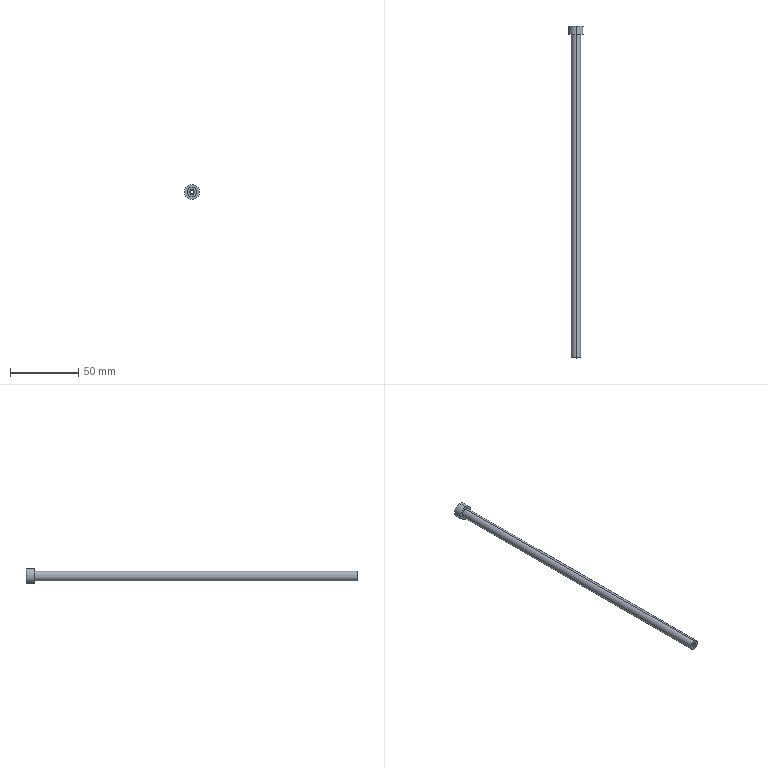Part | STEP file | 1 solid | 12 faces | box 11 x 243.265 x 11 mm | volume 8491 mm3 | cylinder 6 | plane 4 | cone 2 | commonest cylinder face diameters 2.5 x2 7 x2 11 x2
STEP:
#1=CARTESIAN_POINT('',(0.,0.,0.));
#2=DIRECTION('',(0.,0.,1.));
#3=DIRECTION('',(1.,0.,0.));
#4=AXIS2_PLACEMENT_3D('',#1,#2,#3);
#5=CARTESIAN_POINT('',(-72.862,290.5,127.16));
#6=VERTEX_POINT('',#5);
#7=CARTESIAN_POINT('',(-72.862,290.5,138.16));
#8=VERTEX_POINT('',#7);
#9=CARTESIAN_POINT('',(-72.862,290.5,132.66));
#10=DIRECTION('',(0.,-1.,0.));
#11=DIRECTION('',(0.,0.,-1.));
#12=AXIS2_PLACEMENT_3D('',#9,#10,#11);
#13=CIRCLE('',#12,5.5);
#14=CARTESIAN_POINT('',(-72.862,290.5,132.66));
#15=DIRECTION('',(0.,-1.,0.));
#16=DIRECTION('',(0.,0.,-1.));
#17=AXIS2_PLACEMENT_3D('',#14,#15,#16);
#18=CYLINDRICAL_SURFACE('',#17,5.5);
#19=CARTESIAN_POINT('',(0.,0.));
#20=DIRECTION('',(1.,0.));
#21=VECTOR('',#20,1.);
#22=LINE('',#19,#21);
#23=(GEOMETRIC_REPRESENTATION_CONTEXT(2)PARAMETRIC_REPRESENTATION_CONTEXT()REPRESENTATION_CONTEXT('',''));
#24=DEFINITIONAL_REPRESENTATION('',(#22),#23);
#25=PCURVE('',#18,#24);
#26=CARTESIAN_POINT('',(-72.862,290.5,110.196));
#27=DIRECTION('',(0.,-1.,0.));
#28=DIRECTION('',(0.,0.,-1.));
#29=AXIS2_PLACEMENT_3D('',#26,#27,#28);
#30=PLANE('',#29);
#31=CARTESIAN_POINT('',(-22.464,-0.000000011));
#32=DIRECTION('',(1.,0.));
#33=AXIS2_PLACEMENT_2D('',#31,#32);
#34=CIRCLE('',#33,5.5);
#35=(GEOMETRIC_REPRESENTATION_CONTEXT(2)PARAMETRIC_REPRESENTATION_CONTEXT()REPRESENTATION_CONTEXT('',''));
#36=DEFINITIONAL_REPRESENTATION('',(#34),#35);
#37=PCURVE('',#30,#36);
#38=SURFACE_CURVE('',#13,(#25,#37),.PCURVE_S1.);
#39=EDGE_CURVE('',#6,#8,#38,.T.);
#40=ORIENTED_EDGE('',*,*,#39,.T.);
#41=CARTESIAN_POINT('',(-72.862,284.5,138.16));
#42=VERTEX_POINT('',#41);
#43=CARTESIAN_POINT('',(-72.862,290.5,138.16));
#44=DIRECTION('',(0.,-1.,0.));
#45=VECTOR('',#44,1.);
#46=LINE('',#43,#45);
#47=CARTESIAN_POINT('',(3.142,0.));
#48=DIRECTION('',(0.,1.));
#49=VECTOR('',#48,1.);
#50=LINE('',#47,#49);
#51=(GEOMETRIC_REPRESENTATION_CONTEXT(2)PARAMETRIC_REPRESENTATION_CONTEXT()REPRESENTATION_CONTEXT('',''));
#52=DEFINITIONAL_REPRESENTATION('',(#50),#51);
#53=PCURVE('',#18,#52);
#54=CARTESIAN_POINT('',(-72.862,290.5,132.66));
#55=DIRECTION('',(0.,-1.,0.));
#56=DIRECTION('',(0.,0.,-1.));
#57=AXIS2_PLACEMENT_3D('',#54,#55,#56);
#58=CYLINDRICAL_SURFACE('',#57,5.5);
#59=CARTESIAN_POINT('',(3.142,0.));
#60=DIRECTION('',(0.,1.));
#61=VECTOR('',#60,1.);
#62=LINE('',#59,#61);
#63=(GEOMETRIC_REPRESENTATION_CONTEXT(2)PARAMETRIC_REPRESENTATION_CONTEXT()REPRESENTATION_CONTEXT('',''));
#64=DEFINITIONAL_REPRESENTATION('',(#62),#63);
#65=PCURVE('',#58,#64);
#66=SURFACE_CURVE('',#46,(#53,#65),.PCURVE_S1.);
#67=EDGE_CURVE('',#8,#42,#66,.T.);
#68=ORIENTED_EDGE('',*,*,#67,.T.);
#69=CARTESIAN_POINT('',(-72.862,284.5,127.16));
#70=VERTEX_POINT('',#69);
#71=CARTESIAN_POINT('',(-72.862,284.5,132.66));
#72=DIRECTION('',(0.,1.,0.));
#73=DIRECTION('',(0.,0.,1.));
#74=AXIS2_PLACEMENT_3D('',#71,#72,#73);
#75=CIRCLE('',#74,5.5);
#76=CARTESIAN_POINT('',(3.142,6.));
#77=DIRECTION('',(-1.,0.));
#78=VECTOR('',#77,1.);
#79=LINE('',#76,#78);
#80=(GEOMETRIC_REPRESENTATION_CONTEXT(2)PARAMETRIC_REPRESENTATION_CONTEXT()REPRESENTATION_CONTEXT('',''));
#81=DEFINITIONAL_REPRESENTATION('',(#79),#80);
#82=PCURVE('',#18,#81);
#83=CARTESIAN_POINT('',(-72.862,284.5,132.66));
#84=DIRECTION('',(0.,-1.,0.));
#85=DIRECTION('',(0.,0.,-1.));
#86=AXIS2_PLACEMENT_3D('',#83,#84,#85);
#87=PLANE('',#86);
#88=CARTESIAN_POINT('',(-5.5,0.));
#89=CARTESIAN_POINT('',(-5.5,9.526));
#90=CARTESIAN_POINT('',(2.75,4.763));
#91=CARTESIAN_POINT('',(11.,0.));
#92=CARTESIAN_POINT('',(2.75,-4.763));
#93=CARTESIAN_POINT('',(-5.5,-9.526));
#94=CARTESIAN_POINT('',(-5.5,0.));
#95=(BOUNDED_CURVE()B_SPLINE_CURVE(2,(#88,#89,#90,#91,#92,#93,#94),.UNSPECIFIED.,.T.,.F.)B_SPLINE_CURVE_WITH_KNOTS((1,2,2,2,2,1),(-2.094,0.,2.094,4.189,6.283,8.378),.UNSPECIFIED.)CURVE()GEOMETRIC_REPRESENTATION_ITEM()RATIONAL_B_SPLINE_CURVE((1.,0.5,1.,0.5,1.,0.5,1.))REPRESENTATION_ITEM(''));
#96=(GEOMETRIC_REPRESENTATION_CONTEXT(2)PARAMETRIC_REPRESENTATION_CONTEXT()REPRESENTATION_CONTEXT('',''));
#97=DEFINITIONAL_REPRESENTATION('',(#95),#96);
#98=PCURVE('',#87,#97);
#99=SURFACE_CURVE('',#75,(#82,#98),.PCURVE_S1.);
#100=EDGE_CURVE('',#42,#70,#99,.T.);
#101=ORIENTED_EDGE('',*,*,#100,.T.);
#102=CARTESIAN_POINT('',(-72.862,290.5,127.16));
#103=DIRECTION('',(0.,-1.,0.));
#104=VECTOR('',#103,1.);
#105=LINE('',#102,#104);
#106=CARTESIAN_POINT('',(0.,0.));
#107=DIRECTION('',(0.,1.));
#108=VECTOR('',#107,1.);
#109=LINE('',#106,#108);
#110=(GEOMETRIC_REPRESENTATION_CONTEXT(2)PARAMETRIC_REPRESENTATION_CONTEXT()REPRESENTATION_CONTEXT('',''));
#111=DEFINITIONAL_REPRESENTATION('',(#109),#110);
#112=PCURVE('',#18,#111);
#113=CARTESIAN_POINT('',(6.283,0.));
#114=DIRECTION('',(0.,1.));
#115=VECTOR('',#114,1.);
#116=LINE('',#113,#115);
#117=(GEOMETRIC_REPRESENTATION_CONTEXT(2)PARAMETRIC_REPRESENTATION_CONTEXT()REPRESENTATION_CONTEXT('',''));
#118=DEFINITIONAL_REPRESENTATION('',(#116),#117);
#119=PCURVE('',#58,#118);
#120=SURFACE_CURVE('',#105,(#112,#119),.PCURVE_S1.);
#121=EDGE_CURVE('',#6,#70,#120,.T.);
#122=ORIENTED_EDGE('',*,*,#121,.F.);
#123=EDGE_LOOP('',(#40,#68,#101,#122));
#124=FACE_BOUND('',#123,.T.);
#125=ADVANCED_FACE('',(#124),#18,.T.);
#126=CARTESIAN_POINT('',(-72.862,47.235,133.91));
#127=VERTEX_POINT('',#126);
#128=CARTESIAN_POINT('',(-72.862,290.5,133.91));
#129=VERTEX_POINT('',#128);
#130=CARTESIAN_POINT('',(-72.862,39.195,133.91));
#131=DIRECTION('',(0.,1.,0.));
#132=VECTOR('',#131,1.);
#133=LINE('',#130,#132);
#134=CARTESIAN_POINT('',(-72.862,39.195,132.66));
#135=DIRECTION('',(0.,1.,0.));
#136=DIRECTION('',(0.,0.,1.));
#137=AXIS2_PLACEMENT_3D('',#134,#135,#136);
#138=CYLINDRICAL_SURFACE('',#137,1.25);
#139=CARTESIAN_POINT('',(6.283,0.));
#140=DIRECTION('',(0.,1.));
#141=VECTOR('',#140,1.);
#142=LINE('',#139,#141);
#143=(GEOMETRIC_REPRESENTATION_CONTEXT(2)PARAMETRIC_REPRESENTATION_CONTEXT()REPRESENTATION_CONTEXT('',''));
#144=DEFINITIONAL_REPRESENTATION('',(#142),#143);
#145=PCURVE('',#138,#144);
#146=CARTESIAN_POINT('',(-72.862,39.195,132.66));
#147=DIRECTION('',(0.,1.,0.));
#148=DIRECTION('',(0.,0.,1.));
#149=AXIS2_PLACEMENT_3D('',#146,#147,#148);
#150=CYLINDRICAL_SURFACE('',#149,1.25);
#151=CARTESIAN_POINT('',(0.,0.));
#152=DIRECTION('',(0.,1.));
#153=VECTOR('',#152,1.);
#154=LINE('',#151,#153);
#155=(GEOMETRIC_REPRESENTATION_CONTEXT(2)PARAMETRIC_REPRESENTATION_CONTEXT()REPRESENTATION_CONTEXT('',''));
#156=DEFINITIONAL_REPRESENTATION('',(#154),#155);
#157=PCURVE('',#150,#156);
#158=SURFACE_CURVE('',#133,(#145,#157),.PCURVE_S1.);
#159=EDGE_CURVE('',#127,#129,#158,.T.);
#160=ORIENTED_EDGE('',*,*,#159,.T.);
#161=CARTESIAN_POINT('',(-72.862,290.5,131.41));
#162=VERTEX_POINT('',#161);
#163=CARTESIAN_POINT('',(-72.862,290.5,132.66));
#164=DIRECTION('',(0.,-1.,0.));
#165=DIRECTION('',(0.,0.,-1.));
#166=AXIS2_PLACEMENT_3D('',#163,#164,#165);
#167=CIRCLE('',#166,1.25);
#168=CARTESIAN_POINT('',(9.425,251.305));
#169=DIRECTION('',(-1.,0.));
#170=VECTOR('',#169,1.);
#171=LINE('',#168,#170);
#172=(GEOMETRIC_REPRESENTATION_CONTEXT(2)PARAMETRIC_REPRESENTATION_CONTEXT()REPRESENTATION_CONTEXT('',''));
#173=DEFINITIONAL_REPRESENTATION('',(#171),#172);
#174=PCURVE('',#138,#173);
#175=CARTESIAN_POINT('',(-22.464,-0.000000011));
#176=DIRECTION('',(1.,0.));
#177=AXIS2_PLACEMENT_2D('',#175,#176);
#178=CIRCLE('',#177,1.25);
#179=(GEOMETRIC_REPRESENTATION_CONTEXT(2)PARAMETRIC_REPRESENTATION_CONTEXT()REPRESENTATION_CONTEXT('',''));
#180=DEFINITIONAL_REPRESENTATION('',(#178),#179);
#181=PCURVE('',#30,#180);
#182=SURFACE_CURVE('',#167,(#174,#181),.PCURVE_S1.);
#183=EDGE_CURVE('',#129,#162,#182,.T.);
#184=ORIENTED_EDGE('',*,*,#183,.T.);
#185=CARTESIAN_POINT('',(-72.862,47.235,131.41));
#186=VERTEX_POINT('',#185);
#187=CARTESIAN_POINT('',(-72.862,39.195,131.41));
#188=DIRECTION('',(0.,1.,0.));
#189=VECTOR('',#188,1.);
#190=LINE('',#187,#189);
#191=CARTESIAN_POINT('',(3.142,0.));
#192=DIRECTION('',(0.,1.));
#193=VECTOR('',#192,1.);
#194=LINE('',#191,#193);
#195=(GEOMETRIC_REPRESENTATION_CONTEXT(2)PARAMETRIC_REPRESENTATION_CONTEXT()REPRESENTATION_CONTEXT('',''));
#196=DEFINITIONAL_REPRESENTATION('',(#194),#195);
#197=PCURVE('',#138,#196);
#198=CARTESIAN_POINT('',(3.142,0.));
#199=DIRECTION('',(0.,1.));
#200=VECTOR('',#199,1.);
#201=LINE('',#198,#200);
#202=(GEOMETRIC_REPRESENTATION_CONTEXT(2)PARAMETRIC_REPRESENTATION_CONTEXT()REPRESENTATION_CONTEXT('',''));
#203=DEFINITIONAL_REPRESENTATION('',(#201),#202);
#204=PCURVE('',#150,#203);
#205=SURFACE_CURVE('',#190,(#197,#204),.PCURVE_S1.);
#206=EDGE_CURVE('',#186,#162,#205,.T.);
#207=ORIENTED_EDGE('',*,*,#206,.F.);
#208=CARTESIAN_POINT('',(-72.862,47.235,132.66));
#209=DIRECTION('',(0.,-1.,0.));
#210=DIRECTION('',(0.,0.,1.));
#211=AXIS2_PLACEMENT_3D('',#208,#209,#210);
#212=CIRCLE('',#211,1.25);
#213=CARTESIAN_POINT('',(6.283,8.04));
#214=DIRECTION('',(-1.,0.));
#215=VECTOR('',#214,1.);
#216=LINE('',#213,#215);
#217=(GEOMETRIC_REPRESENTATION_CONTEXT(2)PARAMETRIC_REPRESENTATION_CONTEXT()REPRESENTATION_CONTEXT('',''));
#218=DEFINITIONAL_REPRESENTATION('',(#216),#217);
#219=PCURVE('',#138,#218);
#220=CARTESIAN_POINT('',(-72.862,47.235,131.404));
#221=DIRECTION('',(0.,1.,0.));
#222=DIRECTION('',(0.,0.,1.));
#223=AXIS2_PLACEMENT_3D('',#220,#221,#222);
#224=PLANE('',#223);
#225=CARTESIAN_POINT('',(2.506,0.));
#226=CARTESIAN_POINT('',(2.506,-2.165));
#227=CARTESIAN_POINT('',(0.6312,-1.083));
#228=CARTESIAN_POINT('',(-1.244,0.));
#229=CARTESIAN_POINT('',(0.6312,1.083));
#230=CARTESIAN_POINT('',(2.506,2.165));
#231=CARTESIAN_POINT('',(2.506,0.));
#232=(BOUNDED_CURVE()B_SPLINE_CURVE(2,(#225,#226,#227,#228,#229,#230,#231),.UNSPECIFIED.,.T.,.F.)B_SPLINE_CURVE_WITH_KNOTS((1,2,2,2,2,1),(-2.094,0.,2.094,4.189,6.283,8.378),.UNSPECIFIED.)CURVE()GEOMETRIC_REPRESENTATION_ITEM()RATIONAL_B_SPLINE_CURVE((1.,0.5,1.,0.5,1.,0.5,1.))REPRESENTATION_ITEM(''));
#233=(GEOMETRIC_REPRESENTATION_CONTEXT(2)PARAMETRIC_REPRESENTATION_CONTEXT()REPRESENTATION_CONTEXT('',''));
#234=DEFINITIONAL_REPRESENTATION('',(#232),#233);
#235=PCURVE('',#224,#234);
#236=SURFACE_CURVE('',#212,(#219,#235),.PCURVE_S1.);
#237=EDGE_CURVE('',#127,#186,#236,.T.);
#238=ORIENTED_EDGE('',*,*,#237,.F.);
#239=EDGE_LOOP('',(#160,#184,#207,#238));
#240=FACE_BOUND('',#239,.F.);
#241=ADVANCED_FACE('',(#240),#138,.F.);
#242=CARTESIAN_POINT('',(-72.862,47.737,129.16));
#243=VERTEX_POINT('',#242);
#244=CARTESIAN_POINT('',(-72.862,47.737,136.16));
#245=VERTEX_POINT('',#244);
#246=CARTESIAN_POINT('',(-72.862,47.737,132.66));
#247=DIRECTION('',(0.,-1.,0.));
#248=DIRECTION('',(0.,0.,1.));
#249=AXIS2_PLACEMENT_3D('',#246,#247,#248);
#250=CIRCLE('',#249,3.5);
#251=CARTESIAN_POINT('',(-72.862,39.195,132.66));
#252=DIRECTION('',(0.,1.,0.));
#253=DIRECTION('',(0.,0.,1.));
#254=AXIS2_PLACEMENT_3D('',#251,#252,#253);
#255=CYLINDRICAL_SURFACE('',#254,3.5);
#256=CARTESIAN_POINT('',(6.283,8.543));
#257=DIRECTION('',(-1.,0.));
#258=VECTOR('',#257,1.);
#259=LINE('',#256,#258);
#260=(GEOMETRIC_REPRESENTATION_CONTEXT(2)PARAMETRIC_REPRESENTATION_CONTEXT()REPRESENTATION_CONTEXT('',''));
#261=DEFINITIONAL_REPRESENTATION('',(#259),#260);
#262=PCURVE('',#255,#261);
#263=CARTESIAN_POINT('',(-72.862,47.737,132.66));
#264=DIRECTION('',(0.,1.,0.));
#265=DIRECTION('',(0.,0.,1.));
#266=AXIS2_PLACEMENT_3D('',#263,#264,#265);
#267=PLANE('',#266);
#268=CARTESIAN_POINT('',(3.5,0.));
#269=CARTESIAN_POINT('',(3.5,-6.062));
#270=CARTESIAN_POINT('',(-1.75,-3.031));
#271=CARTESIAN_POINT('',(-7.,0.));
#272=CARTESIAN_POINT('',(-1.75,3.031));
#273=CARTESIAN_POINT('',(3.5,6.062));
#274=CARTESIAN_POINT('',(3.5,0.));
#275=(BOUNDED_CURVE()B_SPLINE_CURVE(2,(#268,#269,#270,#271,#272,#273,#274),.UNSPECIFIED.,.T.,.F.)B_SPLINE_CURVE_WITH_KNOTS((1,2,2,2,2,1),(-2.094,0.,2.094,4.189,6.283,8.378),.UNSPECIFIED.)CURVE()GEOMETRIC_REPRESENTATION_ITEM()RATIONAL_B_SPLINE_CURVE((1.,0.5,1.,0.5,1.,0.5,1.))REPRESENTATION_ITEM(''));
#276=(GEOMETRIC_REPRESENTATION_CONTEXT(2)PARAMETRIC_REPRESENTATION_CONTEXT()REPRESENTATION_CONTEXT('',''));
#277=DEFINITIONAL_REPRESENTATION('',(#275),#276);
#278=PCURVE('',#267,#277);
#279=SURFACE_CURVE('',#250,(#262,#278),.PCURVE_S1.);
#280=EDGE_CURVE('',#243,#245,#279,.T.);
#281=ORIENTED_EDGE('',*,*,#280,.F.);
#282=CARTESIAN_POINT('',(-72.862,284.5,129.16));
#283=VERTEX_POINT('',#282);
#284=CARTESIAN_POINT('',(-72.862,39.195,129.16));
#285=DIRECTION('',(0.,1.,0.));
#286=VECTOR('',#285,1.);
#287=LINE('',#284,#286);
#288=CARTESIAN_POINT('',(3.142,0.));
#289=DIRECTION('',(0.,1.));
#290=VECTOR('',#289,1.);
#291=LINE('',#288,#290);
#292=(GEOMETRIC_REPRESENTATION_CONTEXT(2)PARAMETRIC_REPRESENTATION_CONTEXT()REPRESENTATION_CONTEXT('',''));
#293=DEFINITIONAL_REPRESENTATION('',(#291),#292);
#294=PCURVE('',#255,#293);
#295=CARTESIAN_POINT('',(-72.862,39.195,132.66));
#296=DIRECTION('',(0.,1.,0.));
#297=DIRECTION('',(0.,0.,1.));
#298=AXIS2_PLACEMENT_3D('',#295,#296,#297);
#299=CYLINDRICAL_SURFACE('',#298,3.5);
#300=CARTESIAN_POINT('',(3.142,0.));
#301=DIRECTION('',(0.,1.));
#302=VECTOR('',#301,1.);
#303=LINE('',#300,#302);
#304=(GEOMETRIC_REPRESENTATION_CONTEXT(2)PARAMETRIC_REPRESENTATION_CONTEXT()REPRESENTATION_CONTEXT('',''));
#305=DEFINITIONAL_REPRESENTATION('',(#303),#304);
#306=PCURVE('',#299,#305);
#307=SURFACE_CURVE('',#287,(#294,#306),.PCURVE_S1.);
#308=EDGE_CURVE('',#243,#283,#307,.T.);
#309=ORIENTED_EDGE('',*,*,#308,.T.);
#310=CARTESIAN_POINT('',(-72.862,284.5,136.16));
#311=VERTEX_POINT('',#310);
#312=CARTESIAN_POINT('',(-72.862,284.5,132.66));
#313=DIRECTION('',(0.,1.,0.));
#314=DIRECTION('',(0.,0.,-1.));
#315=AXIS2_PLACEMENT_3D('',#312,#313,#314);
#316=CIRCLE('',#315,3.5);
#317=CARTESIAN_POINT('',(-3.142,245.305));
#318=DIRECTION('',(1.,0.));
#319=VECTOR('',#318,1.);
#320=LINE('',#317,#319);
#321=(GEOMETRIC_REPRESENTATION_CONTEXT(2)PARAMETRIC_REPRESENTATION_CONTEXT()REPRESENTATION_CONTEXT('',''));
#322=DEFINITIONAL_REPRESENTATION('',(#320),#321);
#323=PCURVE('',#255,#322);
#324=CARTESIAN_POINT('',(3.5,0.));
#325=CARTESIAN_POINT('',(3.5,-6.062));
#326=CARTESIAN_POINT('',(-1.75,-3.031));
#327=CARTESIAN_POINT('',(-7.,0.));
#328=CARTESIAN_POINT('',(-1.75,3.031));
#329=CARTESIAN_POINT('',(3.5,6.062));
#330=CARTESIAN_POINT('',(3.5,0.));
#331=(BOUNDED_CURVE()B_SPLINE_CURVE(2,(#324,#325,#326,#327,#328,#329,#330),.UNSPECIFIED.,.T.,.F.)B_SPLINE_CURVE_WITH_KNOTS((1,2,2,2,2,1),(-2.094,0.,2.094,4.189,6.283,8.378),.UNSPECIFIED.)CURVE()GEOMETRIC_REPRESENTATION_ITEM()RATIONAL_B_SPLINE_CURVE((1.,0.5,1.,0.5,1.,0.5,1.))REPRESENTATION_ITEM(''));
#332=(GEOMETRIC_REPRESENTATION_CONTEXT(2)PARAMETRIC_REPRESENTATION_CONTEXT()REPRESENTATION_CONTEXT('',''));
#333=DEFINITIONAL_REPRESENTATION('',(#331),#332);
#334=PCURVE('',#87,#333);
#335=SURFACE_CURVE('',#316,(#323,#334),.PCURVE_S1.);
#336=EDGE_CURVE('',#311,#283,#335,.T.);
#337=ORIENTED_EDGE('',*,*,#336,.F.);
#338=CARTESIAN_POINT('',(-72.862,39.195,136.16));
#339=DIRECTION('',(0.,1.,0.));
#340=VECTOR('',#339,1.);
#341=LINE('',#338,#340);
#342=CARTESIAN_POINT('',(0.,0.));
#343=DIRECTION('',(0.,1.));
#344=VECTOR('',#343,1.);
#345=LINE('',#342,#344);
#346=(GEOMETRIC_REPRESENTATION_CONTEXT(2)PARAMETRIC_REPRESENTATION_CONTEXT()REPRESENTATION_CONTEXT('',''));
#347=DEFINITIONAL_REPRESENTATION('',(#345),#346);
#348=PCURVE('',#255,#347);
#349=CARTESIAN_POINT('',(6.283,0.));
#350=DIRECTION('',(0.,1.));
#351=VECTOR('',#350,1.);
#352=LINE('',#349,#351);
#353=(GEOMETRIC_REPRESENTATION_CONTEXT(2)PARAMETRIC_REPRESENTATION_CONTEXT()REPRESENTATION_CONTEXT('',''));
#354=DEFINITIONAL_REPRESENTATION('',(#352),#353);
#355=PCURVE('',#299,#354);
#356=SURFACE_CURVE('',#341,(#348,#355),.PCURVE_S1.);
#357=EDGE_CURVE('',#245,#311,#356,.T.);
#358=ORIENTED_EDGE('',*,*,#357,.F.);
#359=EDGE_LOOP('',(#281,#309,#337,#358));
#360=FACE_BOUND('',#359,.T.);
#361=ADVANCED_FACE('',(#360),#255,.T.);
#362=CARTESIAN_POINT('',(-72.862,47.235,133.916));
#363=VERTEX_POINT('',#362);
#364=CARTESIAN_POINT('',(-72.862,47.235,131.404));
#365=VERTEX_POINT('',#364);
#366=CARTESIAN_POINT('',(-72.862,47.235,132.66));
#367=DIRECTION('',(0.,1.,0.));
#368=DIRECTION('',(0.,0.,1.));
#369=AXIS2_PLACEMENT_3D('',#366,#367,#368);
#370=CIRCLE('',#369,1.256);
#371=CARTESIAN_POINT('',(-72.862,47.235,132.66));
#372=DIRECTION('',(0.,1.,0.));
#373=DIRECTION('',(0.,0.,1.));
#374=AXIS2_PLACEMENT_3D('',#371,#372,#373);
#375=CONICAL_SURFACE('',#374,1.256,0.7854);
#376=CARTESIAN_POINT('',(0.,0.));
#377=DIRECTION('',(1.,0.));
#378=VECTOR('',#377,1.);
#379=LINE('',#376,#378);
#380=(GEOMETRIC_REPRESENTATION_CONTEXT(2)PARAMETRIC_REPRESENTATION_CONTEXT()REPRESENTATION_CONTEXT('',''));
#381=DEFINITIONAL_REPRESENTATION('',(#379),#380);
#382=PCURVE('',#375,#381);
#383=CARTESIAN_POINT('',(1.256,0.));
#384=DIRECTION('',(1.,0.));
#385=AXIS2_PLACEMENT_2D('',#383,#384);
#386=CIRCLE('',#385,1.256);
#387=(GEOMETRIC_REPRESENTATION_CONTEXT(2)PARAMETRIC_REPRESENTATION_CONTEXT()REPRESENTATION_CONTEXT('',''));
#388=DEFINITIONAL_REPRESENTATION('',(#386),#387);
#389=PCURVE('',#224,#388);
#390=SURFACE_CURVE('',#370,(#382,#389),.PCURVE_S1.);
#391=EDGE_CURVE('',#363,#365,#390,.T.);
#392=ORIENTED_EDGE('',*,*,#391,.T.);
#393=CARTESIAN_POINT('',(-72.862,47.737,130.901));
#394=VERTEX_POINT('',#393);
#395=CARTESIAN_POINT('',(-72.862,47.235,131.404));
#396=DIRECTION('',(0.,0.7071,-0.7071));
#397=VECTOR('',#396,1.);
#398=LINE('',#395,#397);
#399=CARTESIAN_POINT('',(3.142,0.));
#400=DIRECTION('',(0.,1.));
#401=VECTOR('',#400,1.);
#402=LINE('',#399,#401);
#403=(GEOMETRIC_REPRESENTATION_CONTEXT(2)PARAMETRIC_REPRESENTATION_CONTEXT()REPRESENTATION_CONTEXT('',''));
#404=DEFINITIONAL_REPRESENTATION('',(#402),#403);
#405=PCURVE('',#375,#404);
#406=CARTESIAN_POINT('',(-72.862,47.235,132.66));
#407=DIRECTION('',(0.,1.,0.));
#408=DIRECTION('',(0.,0.,1.));
#409=AXIS2_PLACEMENT_3D('',#406,#407,#408);
#410=CONICAL_SURFACE('',#409,1.256,0.7854);
#411=CARTESIAN_POINT('',(3.142,0.));
#412=DIRECTION('',(0.,1.));
#413=VECTOR('',#412,1.);
#414=LINE('',#411,#413);
#415=(GEOMETRIC_REPRESENTATION_CONTEXT(2)PARAMETRIC_REPRESENTATION_CONTEXT()REPRESENTATION_CONTEXT('',''));
#416=DEFINITIONAL_REPRESENTATION('',(#414),#415);
#417=PCURVE('',#410,#416);
#418=SURFACE_CURVE('',#398,(#405,#417),.PCURVE_S1.);
#419=EDGE_CURVE('',#365,#394,#418,.T.);
#420=ORIENTED_EDGE('',*,*,#419,.T.);
#421=CARTESIAN_POINT('',(-72.862,47.737,134.419));
#422=VERTEX_POINT('',#421);
#423=CARTESIAN_POINT('',(-72.862,47.737,132.66));
#424=DIRECTION('',(0.,-1.,0.));
#425=DIRECTION('',(0.,0.,1.));
#426=AXIS2_PLACEMENT_3D('',#423,#424,#425);
#427=CIRCLE('',#426,1.759);
#428=CARTESIAN_POINT('',(6.283,0.5025));
#429=DIRECTION('',(-1.,0.));
#430=VECTOR('',#429,1.);
#431=LINE('',#428,#430);
#432=(GEOMETRIC_REPRESENTATION_CONTEXT(2)PARAMETRIC_REPRESENTATION_CONTEXT()REPRESENTATION_CONTEXT('',''));
#433=DEFINITIONAL_REPRESENTATION('',(#431),#432);
#434=PCURVE('',#375,#433);
#435=CARTESIAN_POINT('',(1.759,0.));
#436=CARTESIAN_POINT('',(1.759,-3.046));
#437=CARTESIAN_POINT('',(-0.8794,-1.523));
#438=CARTESIAN_POINT('',(-3.518,0.));
#439=CARTESIAN_POINT('',(-0.8794,1.523));
#440=CARTESIAN_POINT('',(1.759,3.046));
#441=CARTESIAN_POINT('',(1.759,0.));
#442=(BOUNDED_CURVE()B_SPLINE_CURVE(2,(#435,#436,#437,#438,#439,#440,#441),.UNSPECIFIED.,.T.,.F.)B_SPLINE_CURVE_WITH_KNOTS((1,2,2,2,2,1),(-2.094,0.,2.094,4.189,6.283,8.378),.UNSPECIFIED.)CURVE()GEOMETRIC_REPRESENTATION_ITEM()RATIONAL_B_SPLINE_CURVE((1.,0.5,1.,0.5,1.,0.5,1.))REPRESENTATION_ITEM(''));
#443=(GEOMETRIC_REPRESENTATION_CONTEXT(2)PARAMETRIC_REPRESENTATION_CONTEXT()REPRESENTATION_CONTEXT('',''));
#444=DEFINITIONAL_REPRESENTATION('',(#442),#443);
#445=PCURVE('',#267,#444);
#446=SURFACE_CURVE('',#427,(#434,#445),.PCURVE_S1.);
#447=EDGE_CURVE('',#394,#422,#446,.T.);
#448=ORIENTED_EDGE('',*,*,#447,.T.);
#449=CARTESIAN_POINT('',(-72.862,47.235,133.916));
#450=DIRECTION('',(0.,0.7071,0.7071));
#451=VECTOR('',#450,1.);
#452=LINE('',#449,#451);
#453=CARTESIAN_POINT('',(0.,0.));
#454=DIRECTION('',(0.,1.));
#455=VECTOR('',#454,1.);
#456=LINE('',#453,#455);
#457=(GEOMETRIC_REPRESENTATION_CONTEXT(2)PARAMETRIC_REPRESENTATION_CONTEXT()REPRESENTATION_CONTEXT('',''));
#458=DEFINITIONAL_REPRESENTATION('',(#456),#457);
#459=PCURVE('',#375,#458);
#460=CARTESIAN_POINT('',(6.283,0.));
#461=DIRECTION('',(0.,1.));
#462=VECTOR('',#461,1.);
#463=LINE('',#460,#462);
#464=(GEOMETRIC_REPRESENTATION_CONTEXT(2)PARAMETRIC_REPRESENTATION_CONTEXT()REPRESENTATION_CONTEXT('',''));
#465=DEFINITIONAL_REPRESENTATION('',(#463),#464);
#466=PCURVE('',#410,#465);
#467=SURFACE_CURVE('',#452,(#459,#466),.PCURVE_S1.);
#468=EDGE_CURVE('',#363,#422,#467,.T.);
#469=ORIENTED_EDGE('',*,*,#468,.F.);
#470=EDGE_LOOP('',(#392,#420,#448,#469));
#471=FACE_BOUND('',#470,.T.);
#472=ADVANCED_FACE('',(#471),#375,.T.);
#473=ORIENTED_EDGE('',*,*,#419,.F.);
#474=CARTESIAN_POINT('',(-72.862,47.235,132.66));
#475=DIRECTION('',(0.,1.,0.));
#476=DIRECTION('',(0.,0.,1.));
#477=AXIS2_PLACEMENT_3D('',#474,#475,#476);
#478=CIRCLE('',#477,1.256);
#479=CARTESIAN_POINT('',(0.,0.));
#480=DIRECTION('',(1.,0.));
#481=VECTOR('',#480,1.);
#482=LINE('',#479,#481);
#483=(GEOMETRIC_REPRESENTATION_CONTEXT(2)PARAMETRIC_REPRESENTATION_CONTEXT()REPRESENTATION_CONTEXT('',''));
#484=DEFINITIONAL_REPRESENTATION('',(#482),#483);
#485=PCURVE('',#410,#484);
#486=CARTESIAN_POINT('',(1.256,0.));
#487=DIRECTION('',(1.,0.));
#488=AXIS2_PLACEMENT_2D('',#486,#487);
#489=CIRCLE('',#488,1.256);
#490=(GEOMETRIC_REPRESENTATION_CONTEXT(2)PARAMETRIC_REPRESENTATION_CONTEXT()REPRESENTATION_CONTEXT('',''));
#491=DEFINITIONAL_REPRESENTATION('',(#489),#490);
#492=PCURVE('',#224,#491);
#493=SURFACE_CURVE('',#478,(#485,#492),.PCURVE_S1.);
#494=EDGE_CURVE('',#365,#363,#493,.T.);
#495=ORIENTED_EDGE('',*,*,#494,.T.);
#496=ORIENTED_EDGE('',*,*,#468,.T.);
#497=CARTESIAN_POINT('',(-72.862,47.737,132.66));
#498=DIRECTION('',(0.,-1.,0.));
#499=DIRECTION('',(0.,0.,1.));
#500=AXIS2_PLACEMENT_3D('',#497,#498,#499);
#501=CIRCLE('',#500,1.759);
#502=CARTESIAN_POINT('',(6.283,0.5025));
#503=DIRECTION('',(-1.,0.));
#504=VECTOR('',#503,1.);
#505=LINE('',#502,#504);
#506=(GEOMETRIC_REPRESENTATION_CONTEXT(2)PARAMETRIC_REPRESENTATION_CONTEXT()REPRESENTATION_CONTEXT('',''));
#507=DEFINITIONAL_REPRESENTATION('',(#505),#506);
#508=PCURVE('',#410,#507);
#509=CARTESIAN_POINT('',(1.759,0.));
#510=CARTESIAN_POINT('',(1.759,-3.046));
#511=CARTESIAN_POINT('',(-0.8794,-1.523));
#512=CARTESIAN_POINT('',(-3.518,0.));
#513=CARTESIAN_POINT('',(-0.8794,1.523));
#514=CARTESIAN_POINT('',(1.759,3.046));
#515=CARTESIAN_POINT('',(1.759,0.));
#516=(BOUNDED_CURVE()B_SPLINE_CURVE(2,(#509,#510,#511,#512,#513,#514,#515),.UNSPECIFIED.,.T.,.F.)B_SPLINE_CURVE_WITH_KNOTS((1,2,2,2,2,1),(-2.094,0.,2.094,4.189,6.283,8.378),.UNSPECIFIED.)CURVE()GEOMETRIC_REPRESENTATION_ITEM()RATIONAL_B_SPLINE_CURVE((1.,0.5,1.,0.5,1.,0.5,1.))REPRESENTATION_ITEM(''));
#517=(GEOMETRIC_REPRESENTATION_CONTEXT(2)PARAMETRIC_REPRESENTATION_CONTEXT()REPRESENTATION_CONTEXT('',''));
#518=DEFINITIONAL_REPRESENTATION('',(#516),#517);
#519=PCURVE('',#267,#518);
#520=SURFACE_CURVE('',#501,(#508,#519),.PCURVE_S1.);
#521=EDGE_CURVE('',#422,#394,#520,.T.);
#522=ORIENTED_EDGE('',*,*,#521,.T.);
#523=EDGE_LOOP('',(#473,#495,#496,#522));
#524=FACE_BOUND('',#523,.T.);
#525=ADVANCED_FACE('',(#524),#410,.T.);
#526=CARTESIAN_POINT('',(-72.862,47.737,132.66));
#527=DIRECTION('',(0.,-1.,0.));
#528=DIRECTION('',(0.,0.,1.));
#529=AXIS2_PLACEMENT_3D('',#526,#527,#528);
#530=CIRCLE('',#529,3.5);
#531=CARTESIAN_POINT('',(3.5,0.));
#532=CARTESIAN_POINT('',(3.5,-6.062));
#533=CARTESIAN_POINT('',(-1.75,-3.031));
#534=CARTESIAN_POINT('',(-7.,0.));
#535=CARTESIAN_POINT('',(-1.75,3.031));
#536=CARTESIAN_POINT('',(3.5,6.062));
#537=CARTESIAN_POINT('',(3.5,0.));
#538=(BOUNDED_CURVE()B_SPLINE_CURVE(2,(#531,#532,#533,#534,#535,#536,#537),.UNSPECIFIED.,.T.,.F.)B_SPLINE_CURVE_WITH_KNOTS((1,2,2,2,2,1),(-2.094,0.,2.094,4.189,6.283,8.378),.UNSPECIFIED.)CURVE()GEOMETRIC_REPRESENTATION_ITEM()RATIONAL_B_SPLINE_CURVE((1.,0.5,1.,0.5,1.,0.5,1.))REPRESENTATION_ITEM(''));
#539=(GEOMETRIC_REPRESENTATION_CONTEXT(2)PARAMETRIC_REPRESENTATION_CONTEXT()REPRESENTATION_CONTEXT('',''));
#540=DEFINITIONAL_REPRESENTATION('',(#538),#539);
#541=PCURVE('',#267,#540);
#542=CARTESIAN_POINT('',(6.283,8.543));
#543=DIRECTION('',(-1.,0.));
#544=VECTOR('',#543,1.);
#545=LINE('',#542,#544);
#546=(GEOMETRIC_REPRESENTATION_CONTEXT(2)PARAMETRIC_REPRESENTATION_CONTEXT()REPRESENTATION_CONTEXT('',''));
#547=DEFINITIONAL_REPRESENTATION('',(#545),#546);
#548=PCURVE('',#299,#547);
#549=SURFACE_CURVE('',#530,(#541,#548),.PCURVE_S1.);
#550=EDGE_CURVE('',#245,#243,#549,.T.);
#551=ORIENTED_EDGE('',*,*,#550,.T.);
#552=ORIENTED_EDGE('',*,*,#280,.T.);
#553=EDGE_LOOP('',(#551,#552));
#554=FACE_BOUND('',#553,.T.);
#555=ORIENTED_EDGE('',*,*,#521,.F.);
#556=ORIENTED_EDGE('',*,*,#447,.F.);
#557=EDGE_LOOP('',(#555,#556));
#558=FACE_BOUND('',#557,.T.);
#559=ADVANCED_FACE('',(#554,#558),#267,.F.);
#560=ORIENTED_EDGE('',*,*,#308,.F.);
#561=ORIENTED_EDGE('',*,*,#550,.F.);
#562=ORIENTED_EDGE('',*,*,#357,.T.);
#563=CARTESIAN_POINT('',(-72.862,284.5,132.66));
#564=DIRECTION('',(0.,1.,0.));
#565=DIRECTION('',(0.,0.,-1.));
#566=AXIS2_PLACEMENT_3D('',#563,#564,#565);
#567=CIRCLE('',#566,3.5);
#568=CARTESIAN_POINT('',(3.142,245.305));
#569=DIRECTION('',(1.,0.));
#570=VECTOR('',#569,1.);
#571=LINE('',#568,#570);
#572=(GEOMETRIC_REPRESENTATION_CONTEXT(2)PARAMETRIC_REPRESENTATION_CONTEXT()REPRESENTATION_CONTEXT('',''));
#573=DEFINITIONAL_REPRESENTATION('',(#571),#572);
#574=PCURVE('',#299,#573);
#575=CARTESIAN_POINT('',(3.5,0.));
#576=CARTESIAN_POINT('',(3.5,-6.062));
#577=CARTESIAN_POINT('',(-1.75,-3.031));
#578=CARTESIAN_POINT('',(-7.,0.));
#579=CARTESIAN_POINT('',(-1.75,3.031));
#580=CARTESIAN_POINT('',(3.5,6.062));
#581=CARTESIAN_POINT('',(3.5,0.));
#582=(BOUNDED_CURVE()B_SPLINE_CURVE(2,(#575,#576,#577,#578,#579,#580,#581),.UNSPECIFIED.,.T.,.F.)B_SPLINE_CURVE_WITH_KNOTS((1,2,2,2,2,1),(-2.094,0.,2.094,4.189,6.283,8.378),.UNSPECIFIED.)CURVE()GEOMETRIC_REPRESENTATION_ITEM()RATIONAL_B_SPLINE_CURVE((1.,0.5,1.,0.5,1.,0.5,1.))REPRESENTATION_ITEM(''));
#583=(GEOMETRIC_REPRESENTATION_CONTEXT(2)PARAMETRIC_REPRESENTATION_CONTEXT()REPRESENTATION_CONTEXT('',''));
#584=DEFINITIONAL_REPRESENTATION('',(#582),#583);
#585=PCURVE('',#87,#584);
#586=SURFACE_CURVE('',#567,(#574,#585),.PCURVE_S1.);
#587=EDGE_CURVE('',#283,#311,#586,.T.);
#588=ORIENTED_EDGE('',*,*,#587,.F.);
#589=EDGE_LOOP('',(#560,#561,#562,#588));
#590=FACE_BOUND('',#589,.T.);
#591=ADVANCED_FACE('',(#590),#299,.T.);
#592=CARTESIAN_POINT('',(-72.862,290.5,132.66));
#593=DIRECTION('',(0.,-1.,0.));
#594=DIRECTION('',(0.,0.,-1.));
#595=AXIS2_PLACEMENT_3D('',#592,#593,#594);
#596=CIRCLE('',#595,1.25);
#597=CARTESIAN_POINT('',(3.142,251.305));
#598=DIRECTION('',(-1.,0.));
#599=VECTOR('',#598,1.);
#600=LINE('',#597,#599);
#601=(GEOMETRIC_REPRESENTATION_CONTEXT(2)PARAMETRIC_REPRESENTATION_CONTEXT()REPRESENTATION_CONTEXT('',''));
#602=DEFINITIONAL_REPRESENTATION('',(#600),#601);
#603=PCURVE('',#150,#602);
#604=CARTESIAN_POINT('',(-22.464,-0.000000011));
#605=DIRECTION('',(1.,0.));
#606=AXIS2_PLACEMENT_2D('',#604,#605);
#607=CIRCLE('',#606,1.25);
#608=(GEOMETRIC_REPRESENTATION_CONTEXT(2)PARAMETRIC_REPRESENTATION_CONTEXT()REPRESENTATION_CONTEXT('',''));
#609=DEFINITIONAL_REPRESENTATION('',(#607),#608);
#610=PCURVE('',#30,#609);
#611=SURFACE_CURVE('',#596,(#603,#610),.PCURVE_S1.);
#612=EDGE_CURVE('',#162,#129,#611,.T.);
#613=ORIENTED_EDGE('',*,*,#612,.T.);
#614=ORIENTED_EDGE('',*,*,#159,.F.);
#615=CARTESIAN_POINT('',(-72.862,47.235,132.66));
#616=DIRECTION('',(0.,-1.,0.));
#617=DIRECTION('',(0.,0.,1.));
#618=AXIS2_PLACEMENT_3D('',#615,#616,#617);
#619=CIRCLE('',#618,1.25);
#620=CARTESIAN_POINT('',(6.283,8.04));
#621=DIRECTION('',(-1.,0.));
#622=VECTOR('',#621,1.);
#623=LINE('',#620,#622);
#624=(GEOMETRIC_REPRESENTATION_CONTEXT(2)PARAMETRIC_REPRESENTATION_CONTEXT()REPRESENTATION_CONTEXT('',''));
#625=DEFINITIONAL_REPRESENTATION('',(#623),#624);
#626=PCURVE('',#150,#625);
#627=CARTESIAN_POINT('',(2.506,0.));
#628=CARTESIAN_POINT('',(2.506,-2.165));
#629=CARTESIAN_POINT('',(0.6312,-1.083));
#630=CARTESIAN_POINT('',(-1.244,0.));
#631=CARTESIAN_POINT('',(0.6312,1.083));
#632=CARTESIAN_POINT('',(2.506,2.165));
#633=CARTESIAN_POINT('',(2.506,0.));
#634=(BOUNDED_CURVE()B_SPLINE_CURVE(2,(#627,#628,#629,#630,#631,#632,#633),.UNSPECIFIED.,.T.,.F.)B_SPLINE_CURVE_WITH_KNOTS((1,2,2,2,2,1),(-2.094,0.,2.094,4.189,6.283,8.378),.UNSPECIFIED.)CURVE()GEOMETRIC_REPRESENTATION_ITEM()RATIONAL_B_SPLINE_CURVE((1.,0.5,1.,0.5,1.,0.5,1.))REPRESENTATION_ITEM(''));
#635=(GEOMETRIC_REPRESENTATION_CONTEXT(2)PARAMETRIC_REPRESENTATION_CONTEXT()REPRESENTATION_CONTEXT('',''));
#636=DEFINITIONAL_REPRESENTATION('',(#634),#635);
#637=PCURVE('',#224,#636);
#638=SURFACE_CURVE('',#619,(#626,#637),.PCURVE_S1.);
#639=EDGE_CURVE('',#186,#127,#638,.T.);
#640=ORIENTED_EDGE('',*,*,#639,.F.);
#641=ORIENTED_EDGE('',*,*,#206,.T.);
#642=EDGE_LOOP('',(#613,#614,#640,#641));
#643=FACE_BOUND('',#642,.F.);
#644=ADVANCED_FACE('',(#643),#150,.F.);
#645=ORIENTED_EDGE('',*,*,#237,.F.);
#646=ORIENTED_EDGE('',*,*,#639,.F.);
#647=EDGE_LOOP('',(#645,#646));
#648=FACE_BOUND('',#647,.T.);
#649=ORIENTED_EDGE('',*,*,#391,.F.);
#650=ORIENTED_EDGE('',*,*,#494,.F.);
#651=EDGE_LOOP('',(#649,#650));
#652=FACE_BOUND('',#651,.T.);
#653=ADVANCED_FACE('',(#648,#652),#224,.F.);
#654=ORIENTED_EDGE('',*,*,#336,.T.);
#655=ORIENTED_EDGE('',*,*,#587,.T.);
#656=EDGE_LOOP('',(#654,#655));
#657=FACE_BOUND('',#656,.T.);
#658=CARTESIAN_POINT('',(-72.862,284.5,132.66));
#659=DIRECTION('',(0.,1.,0.));
#660=DIRECTION('',(0.,0.,1.));
#661=AXIS2_PLACEMENT_3D('',#658,#659,#660);
#662=CIRCLE('',#661,5.5);
#663=CARTESIAN_POINT('',(-5.5,0.));
#664=CARTESIAN_POINT('',(-5.5,9.526));
#665=CARTESIAN_POINT('',(2.75,4.763));
#666=CARTESIAN_POINT('',(11.,0.));
#667=CARTESIAN_POINT('',(2.75,-4.763));
#668=CARTESIAN_POINT('',(-5.5,-9.526));
#669=CARTESIAN_POINT('',(-5.5,0.));
#670=(BOUNDED_CURVE()B_SPLINE_CURVE(2,(#663,#664,#665,#666,#667,#668,#669),.UNSPECIFIED.,.T.,.F.)B_SPLINE_CURVE_WITH_KNOTS((1,2,2,2,2,1),(-2.094,0.,2.094,4.189,6.283,8.378),.UNSPECIFIED.)CURVE()GEOMETRIC_REPRESENTATION_ITEM()RATIONAL_B_SPLINE_CURVE((1.,0.5,1.,0.5,1.,0.5,1.))REPRESENTATION_ITEM(''));
#671=(GEOMETRIC_REPRESENTATION_CONTEXT(2)PARAMETRIC_REPRESENTATION_CONTEXT()REPRESENTATION_CONTEXT('',''));
#672=DEFINITIONAL_REPRESENTATION('',(#670),#671);
#673=PCURVE('',#87,#672);
#674=CARTESIAN_POINT('',(9.425,6.));
#675=DIRECTION('',(-1.,0.));
#676=VECTOR('',#675,1.);
#677=LINE('',#674,#676);
#678=(GEOMETRIC_REPRESENTATION_CONTEXT(2)PARAMETRIC_REPRESENTATION_CONTEXT()REPRESENTATION_CONTEXT('',''));
#679=DEFINITIONAL_REPRESENTATION('',(#677),#678);
#680=PCURVE('',#58,#679);
#681=SURFACE_CURVE('',#662,(#673,#680),.PCURVE_S1.);
#682=EDGE_CURVE('',#70,#42,#681,.T.);
#683=ORIENTED_EDGE('',*,*,#682,.F.);
#684=ORIENTED_EDGE('',*,*,#100,.F.);
#685=EDGE_LOOP('',(#683,#684));
#686=FACE_BOUND('',#685,.T.);
#687=ADVANCED_FACE('',(#657,#686),#87,.T.);
#688=ORIENTED_EDGE('',*,*,#67,.F.);
#689=CARTESIAN_POINT('',(-72.862,290.5,132.66));
#690=DIRECTION('',(0.,-1.,0.));
#691=DIRECTION('',(0.,0.,-1.));
#692=AXIS2_PLACEMENT_3D('',#689,#690,#691);
#693=CIRCLE('',#692,5.5);
#694=CARTESIAN_POINT('',(0.,0.));
#695=DIRECTION('',(1.,0.));
#696=VECTOR('',#695,1.);
#697=LINE('',#694,#696);
#698=(GEOMETRIC_REPRESENTATION_CONTEXT(2)PARAMETRIC_REPRESENTATION_CONTEXT()REPRESENTATION_CONTEXT('',''));
#699=DEFINITIONAL_REPRESENTATION('',(#697),#698);
#700=PCURVE('',#58,#699);
#701=CARTESIAN_POINT('',(-22.464,-0.000000011));
#702=DIRECTION('',(1.,0.));
#703=AXIS2_PLACEMENT_2D('',#701,#702);
#704=CIRCLE('',#703,5.5);
#705=(GEOMETRIC_REPRESENTATION_CONTEXT(2)PARAMETRIC_REPRESENTATION_CONTEXT()REPRESENTATION_CONTEXT('',''));
#706=DEFINITIONAL_REPRESENTATION('',(#704),#705);
#707=PCURVE('',#30,#706);
#708=SURFACE_CURVE('',#693,(#700,#707),.PCURVE_S1.);
#709=EDGE_CURVE('',#8,#6,#708,.T.);
#710=ORIENTED_EDGE('',*,*,#709,.T.);
#711=ORIENTED_EDGE('',*,*,#121,.T.);
#712=ORIENTED_EDGE('',*,*,#682,.T.);
#713=EDGE_LOOP('',(#688,#710,#711,#712));
#714=FACE_BOUND('',#713,.T.);
#715=ADVANCED_FACE('',(#714),#58,.T.);
#716=ORIENTED_EDGE('',*,*,#183,.T.);
#717=ORIENTED_EDGE('',*,*,#612,.T.);
#718=EDGE_LOOP('',(#716,#717));
#719=FACE_BOUND('',#718,.T.);
#720=ORIENTED_EDGE('',*,*,#39,.F.);
#721=ORIENTED_EDGE('',*,*,#709,.F.);
#722=EDGE_LOOP('',(#720,#721));
#723=FACE_BOUND('',#722,.T.);
#724=ADVANCED_FACE('',(#719,#723),#30,.F.);
#725=CLOSED_SHELL('',(#125,#241,#361,#472,#525,#559,#591,#644,#653,#687,#715,#724));
#726=MANIFOLD_SOLID_BREP('',#725);
#727=(LENGTH_UNIT()NAMED_UNIT(*)SI_UNIT(.MILLI.,.METRE.));
#728=UNCERTAINTY_MEASURE_WITH_UNIT(LENGTH_MEASURE(0.0000001),#727,'','');
#729=(NAMED_UNIT(*)PLANE_ANGLE_UNIT()SI_UNIT($,.RADIAN.));
#730=(NAMED_UNIT(*)SI_UNIT($,.STERADIAN.)SOLID_ANGLE_UNIT());
#731=(GEOMETRIC_REPRESENTATION_CONTEXT(3)GLOBAL_UNCERTAINTY_ASSIGNED_CONTEXT((#728))GLOBAL_UNIT_ASSIGNED_CONTEXT((#727,#729,#730))REPRESENTATION_CONTEXT('',''));
#732=ADVANCED_BREP_SHAPE_REPRESENTATION('',(#4,#726),#731);